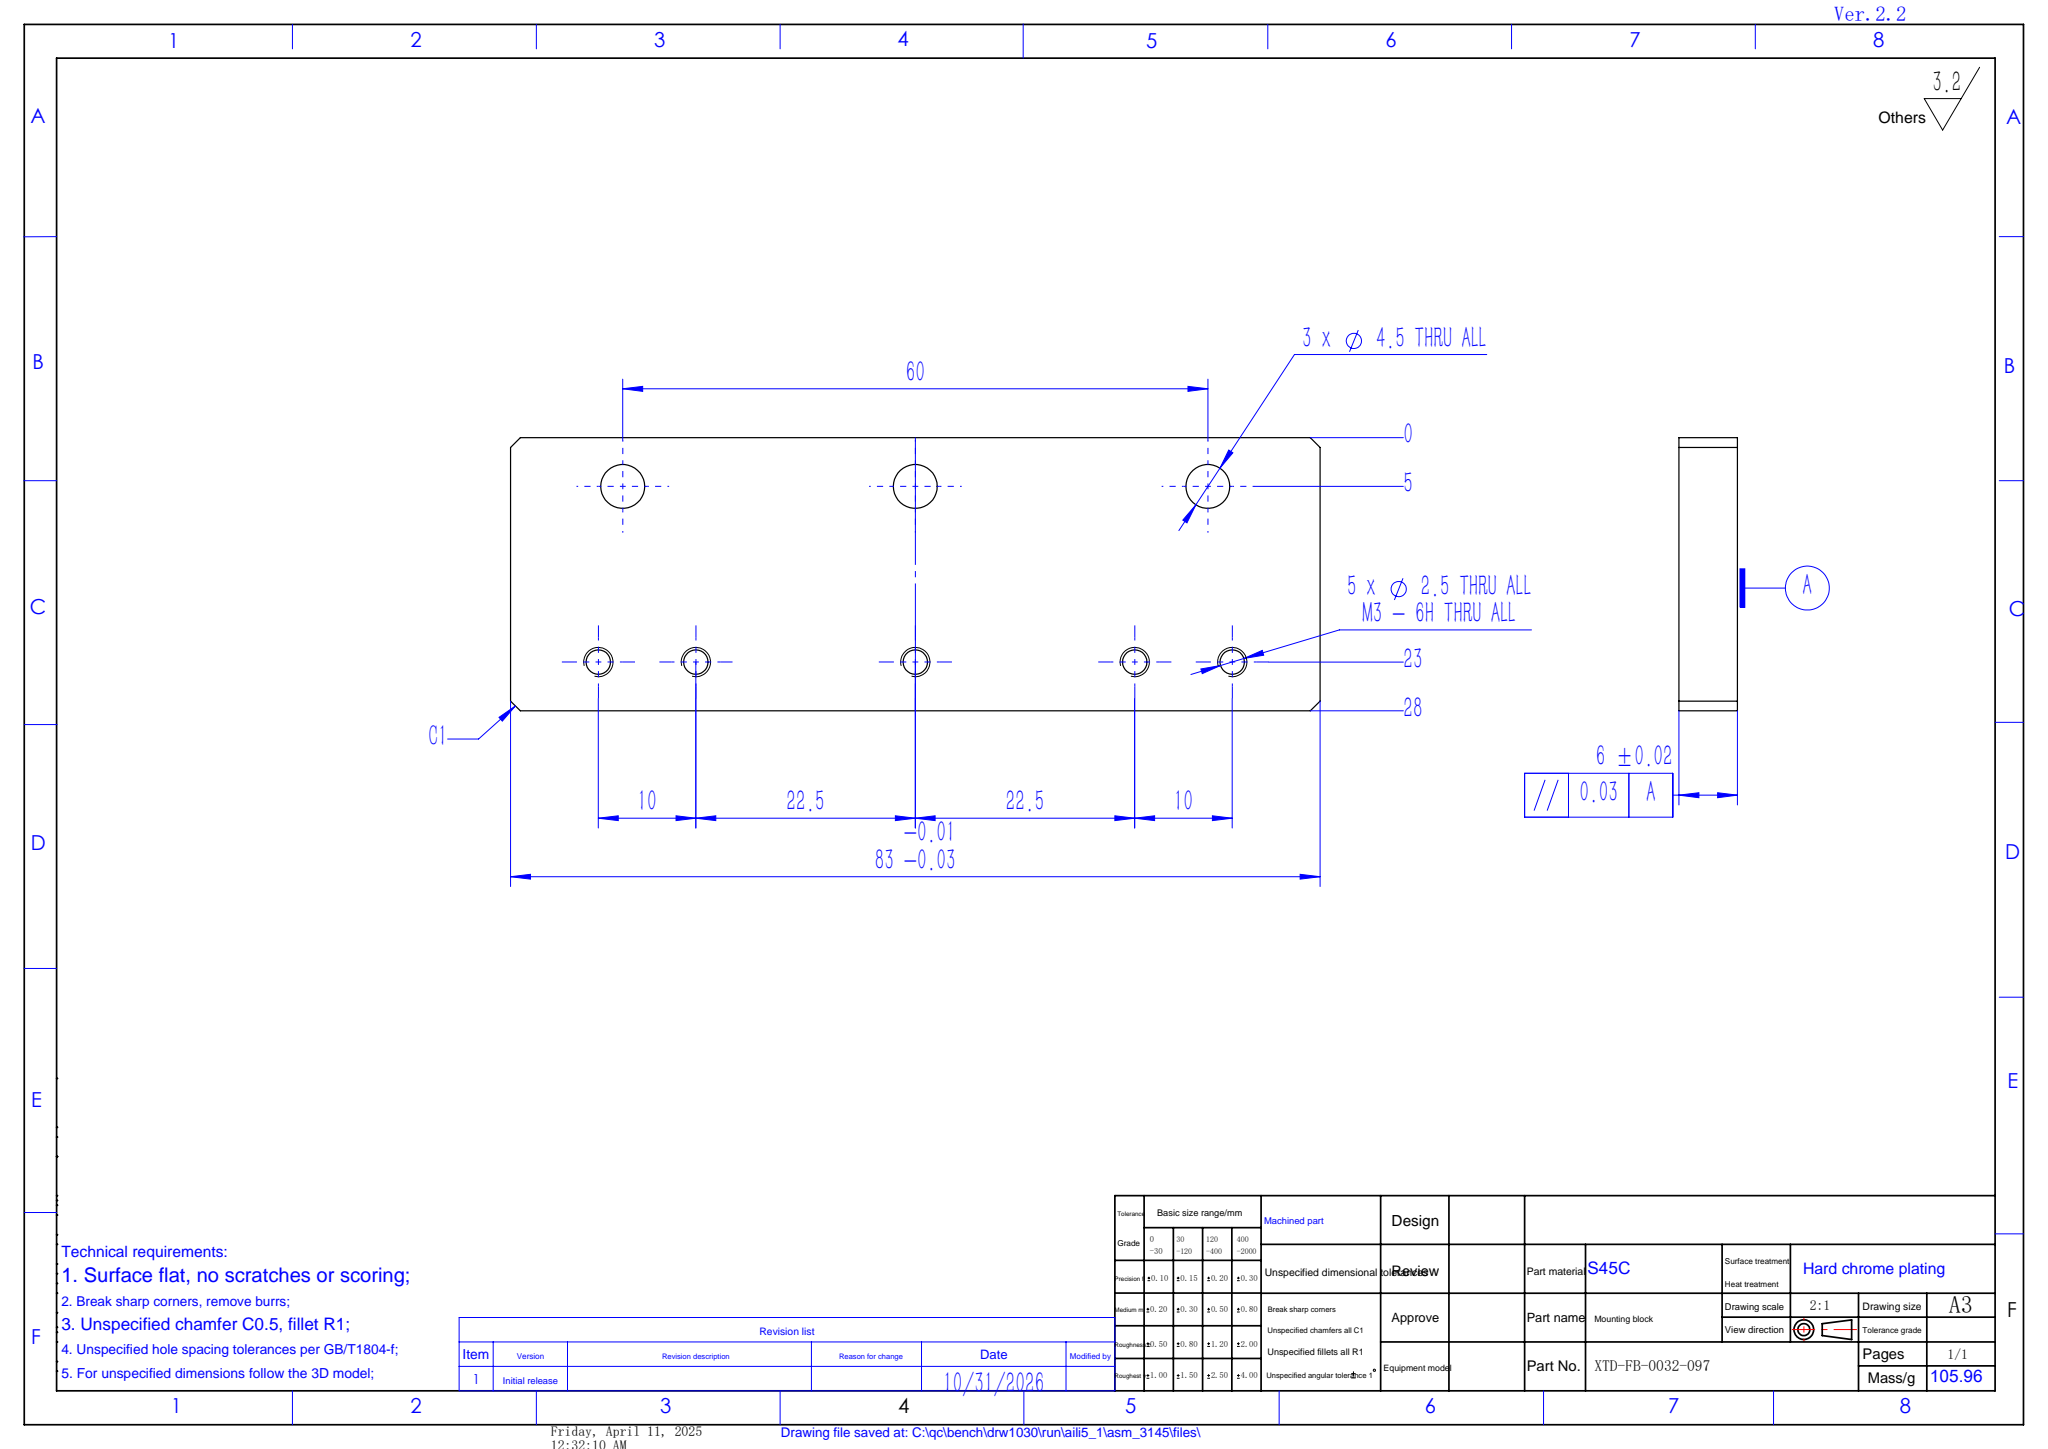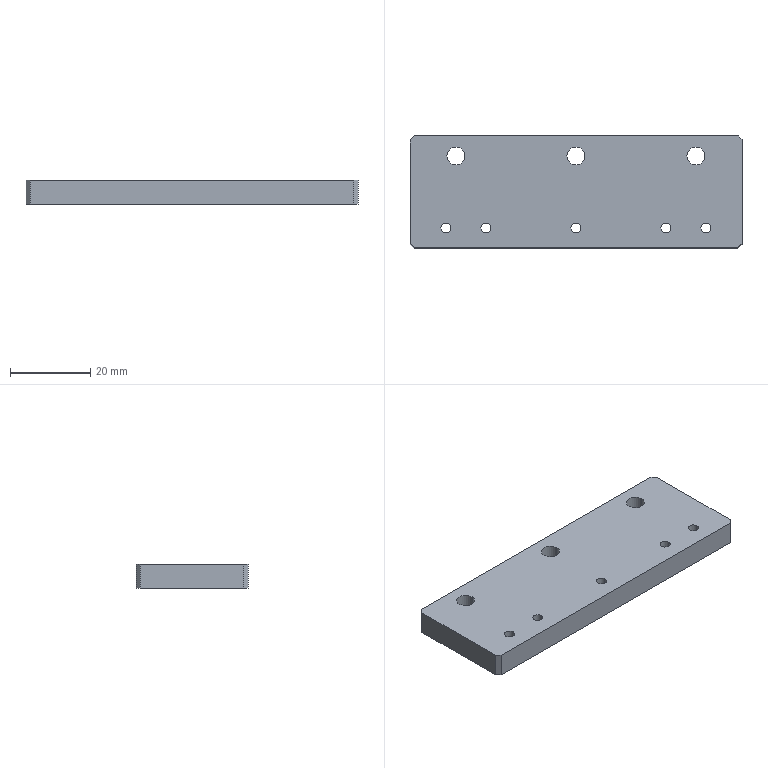Part | SolidWorks | features HoleWzd 2, Chamfer 1, Extrusion 1 | 1 solid | 26 faces | box 83 x 28 x 6 mm | volume 13498 mm3 | cylinder 16 | plane 10 | commonest cylinder face diameters 2.5 x10 4.5 x6
STEP:
#1=CARTESIAN_POINT('',(-33.75,-9.,0.));
#2=VERTEX_POINT('',#1);
#3=CARTESIAN_POINT('',(-31.25,-9.,0.));
#4=VERTEX_POINT('',#3);
#5=CARTESIAN_POINT('',(-32.5,-9.,0.));
#6=DIRECTION('',(0.,0.,1.));
#7=DIRECTION('',(1.,0.,0.));
#8=AXIS2_PLACEMENT_3D('',#5,#6,#7);
#9=CIRCLE('',#8,1.25);
#10=EDGE_CURVE('',#2,#4,#9,.T.);
#11=ORIENTED_EDGE('',*,*,#10,.F.);
#12=CARTESIAN_POINT('',(-33.75,-9.,6.));
#13=VERTEX_POINT('',#12);
#14=CARTESIAN_POINT('',(-33.75,-9.,6.));
#15=DIRECTION('',(0.,0.,1.));
#16=VECTOR('',#15,1000.);
#17=LINE('',#14,#16);
#18=EDGE_CURVE('',#2,#13,#17,.T.);
#19=ORIENTED_EDGE('',*,*,#18,.T.);
#20=CARTESIAN_POINT('',(-31.25,-9.,6.));
#21=VERTEX_POINT('',#20);
#22=CARTESIAN_POINT('',(-32.5,-9.,6.));
#23=DIRECTION('',(0.,0.,1.));
#24=DIRECTION('',(1.,0.,0.));
#25=AXIS2_PLACEMENT_3D('',#22,#23,#24);
#26=CIRCLE('',#25,1.25);
#27=EDGE_CURVE('',#13,#21,#26,.T.);
#28=ORIENTED_EDGE('',*,*,#27,.T.);
#29=CARTESIAN_POINT('',(-31.25,-9.,6.));
#30=DIRECTION('',(0.,0.,1.));
#31=VECTOR('',#30,1000.);
#32=LINE('',#29,#31);
#33=EDGE_CURVE('',#4,#21,#32,.T.);
#34=ORIENTED_EDGE('',*,*,#33,.F.);
#35=EDGE_LOOP('',(#11,#19,#28,#34));
#36=FACE_OUTER_BOUND('',#35,.T.);
#37=CARTESIAN_POINT('',(-32.5,-9.,6.));
#38=DIRECTION('',(0.,0.,1.));
#39=DIRECTION('',(1.,0.,0.));
#40=AXIS2_PLACEMENT_3D('',#37,#38,#39);
#41=CYLINDRICAL_SURFACE('',#40,1.25);
#42=ADVANCED_FACE('',(#36),#41,.F.);
#43=CARTESIAN_POINT('',(-1.25,-9.,0.));
#44=VERTEX_POINT('',#43);
#45=CARTESIAN_POINT('',(1.25,-9.,0.));
#46=VERTEX_POINT('',#45);
#47=CARTESIAN_POINT('',(0.,-9.,0.));
#48=DIRECTION('',(0.,0.,1.));
#49=DIRECTION('',(1.,0.,0.));
#50=AXIS2_PLACEMENT_3D('',#47,#48,#49);
#51=CIRCLE('',#50,1.25);
#52=EDGE_CURVE('',#44,#46,#51,.T.);
#53=ORIENTED_EDGE('',*,*,#52,.F.);
#54=CARTESIAN_POINT('',(-1.25,-9.,6.));
#55=VERTEX_POINT('',#54);
#56=CARTESIAN_POINT('',(-1.25,-9.,6.));
#57=DIRECTION('',(0.,0.,1.));
#58=VECTOR('',#57,1000.);
#59=LINE('',#56,#58);
#60=EDGE_CURVE('',#44,#55,#59,.T.);
#61=ORIENTED_EDGE('',*,*,#60,.T.);
#62=CARTESIAN_POINT('',(1.25,-9.,6.));
#63=VERTEX_POINT('',#62);
#64=CARTESIAN_POINT('',(0.,-9.,6.));
#65=DIRECTION('',(0.,0.,1.));
#66=DIRECTION('',(1.,0.,0.));
#67=AXIS2_PLACEMENT_3D('',#64,#65,#66);
#68=CIRCLE('',#67,1.25);
#69=EDGE_CURVE('',#55,#63,#68,.T.);
#70=ORIENTED_EDGE('',*,*,#69,.T.);
#71=CARTESIAN_POINT('',(1.25,-9.,6.));
#72=DIRECTION('',(0.,0.,1.));
#73=VECTOR('',#72,1000.);
#74=LINE('',#71,#73);
#75=EDGE_CURVE('',#46,#63,#74,.T.);
#76=ORIENTED_EDGE('',*,*,#75,.F.);
#77=EDGE_LOOP('',(#53,#61,#70,#76));
#78=FACE_OUTER_BOUND('',#77,.T.);
#79=CARTESIAN_POINT('',(0.,-9.,6.));
#80=DIRECTION('',(0.,0.,1.));
#81=DIRECTION('',(1.,0.,0.));
#82=AXIS2_PLACEMENT_3D('',#79,#80,#81);
#83=CYLINDRICAL_SURFACE('',#82,1.25);
#84=ADVANCED_FACE('',(#78),#83,.F.);
#85=CARTESIAN_POINT('',(31.25,-9.,0.));
#86=VERTEX_POINT('',#85);
#87=CARTESIAN_POINT('',(33.75,-9.,0.));
#88=VERTEX_POINT('',#87);
#89=CARTESIAN_POINT('',(32.5,-9.,0.));
#90=DIRECTION('',(0.,0.,1.));
#91=DIRECTION('',(1.,0.,0.));
#92=AXIS2_PLACEMENT_3D('',#89,#90,#91);
#93=CIRCLE('',#92,1.25);
#94=EDGE_CURVE('',#86,#88,#93,.T.);
#95=ORIENTED_EDGE('',*,*,#94,.F.);
#96=CARTESIAN_POINT('',(31.25,-9.,6.));
#97=VERTEX_POINT('',#96);
#98=CARTESIAN_POINT('',(31.25,-9.,6.));
#99=DIRECTION('',(0.,0.,1.));
#100=VECTOR('',#99,1000.);
#101=LINE('',#98,#100);
#102=EDGE_CURVE('',#86,#97,#101,.T.);
#103=ORIENTED_EDGE('',*,*,#102,.T.);
#104=CARTESIAN_POINT('',(33.75,-9.,6.));
#105=VERTEX_POINT('',#104);
#106=CARTESIAN_POINT('',(32.5,-9.,6.));
#107=DIRECTION('',(0.,0.,1.));
#108=DIRECTION('',(1.,0.,0.));
#109=AXIS2_PLACEMENT_3D('',#106,#107,#108);
#110=CIRCLE('',#109,1.25);
#111=EDGE_CURVE('',#97,#105,#110,.T.);
#112=ORIENTED_EDGE('',*,*,#111,.T.);
#113=CARTESIAN_POINT('',(33.75,-9.,6.));
#114=DIRECTION('',(0.,0.,1.));
#115=VECTOR('',#114,1000.);
#116=LINE('',#113,#115);
#117=EDGE_CURVE('',#88,#105,#116,.T.);
#118=ORIENTED_EDGE('',*,*,#117,.F.);
#119=EDGE_LOOP('',(#95,#103,#112,#118));
#120=FACE_OUTER_BOUND('',#119,.T.);
#121=CARTESIAN_POINT('',(32.5,-9.,6.));
#122=DIRECTION('',(0.,0.,1.));
#123=DIRECTION('',(1.,0.,0.));
#124=AXIS2_PLACEMENT_3D('',#121,#122,#123);
#125=CYLINDRICAL_SURFACE('',#124,1.25);
#126=ADVANCED_FACE('',(#120),#125,.F.);
#127=CARTESIAN_POINT('',(21.25,-9.,0.));
#128=VERTEX_POINT('',#127);
#129=CARTESIAN_POINT('',(23.75,-9.,0.));
#130=VERTEX_POINT('',#129);
#131=CARTESIAN_POINT('',(22.5,-9.,0.));
#132=DIRECTION('',(0.,0.,1.));
#133=DIRECTION('',(1.,0.,0.));
#134=AXIS2_PLACEMENT_3D('',#131,#132,#133);
#135=CIRCLE('',#134,1.25);
#136=EDGE_CURVE('',#128,#130,#135,.T.);
#137=ORIENTED_EDGE('',*,*,#136,.F.);
#138=CARTESIAN_POINT('',(21.25,-9.,6.));
#139=VERTEX_POINT('',#138);
#140=CARTESIAN_POINT('',(21.25,-9.,6.));
#141=DIRECTION('',(0.,0.,1.));
#142=VECTOR('',#141,1000.);
#143=LINE('',#140,#142);
#144=EDGE_CURVE('',#128,#139,#143,.T.);
#145=ORIENTED_EDGE('',*,*,#144,.T.);
#146=CARTESIAN_POINT('',(23.75,-9.,6.));
#147=VERTEX_POINT('',#146);
#148=CARTESIAN_POINT('',(22.5,-9.,6.));
#149=DIRECTION('',(0.,0.,1.));
#150=DIRECTION('',(1.,0.,0.));
#151=AXIS2_PLACEMENT_3D('',#148,#149,#150);
#152=CIRCLE('',#151,1.25);
#153=EDGE_CURVE('',#139,#147,#152,.T.);
#154=ORIENTED_EDGE('',*,*,#153,.T.);
#155=CARTESIAN_POINT('',(23.75,-9.,6.));
#156=DIRECTION('',(0.,0.,1.));
#157=VECTOR('',#156,1000.);
#158=LINE('',#155,#157);
#159=EDGE_CURVE('',#130,#147,#158,.T.);
#160=ORIENTED_EDGE('',*,*,#159,.F.);
#161=EDGE_LOOP('',(#137,#145,#154,#160));
#162=FACE_OUTER_BOUND('',#161,.T.);
#163=CARTESIAN_POINT('',(22.5,-9.,6.));
#164=DIRECTION('',(0.,0.,1.));
#165=DIRECTION('',(1.,0.,0.));
#166=AXIS2_PLACEMENT_3D('',#163,#164,#165);
#167=CYLINDRICAL_SURFACE('',#166,1.25);
#168=ADVANCED_FACE('',(#162),#167,.F.);
#169=CARTESIAN_POINT('',(-23.75,-9.,0.));
#170=VERTEX_POINT('',#169);
#171=CARTESIAN_POINT('',(-21.25,-9.,0.));
#172=VERTEX_POINT('',#171);
#173=CARTESIAN_POINT('',(-22.5,-9.,0.));
#174=DIRECTION('',(0.,0.,1.));
#175=DIRECTION('',(1.,0.,0.));
#176=AXIS2_PLACEMENT_3D('',#173,#174,#175);
#177=CIRCLE('',#176,1.25);
#178=EDGE_CURVE('',#170,#172,#177,.T.);
#179=ORIENTED_EDGE('',*,*,#178,.F.);
#180=CARTESIAN_POINT('',(-23.75,-9.,6.));
#181=VERTEX_POINT('',#180);
#182=CARTESIAN_POINT('',(-23.75,-9.,6.));
#183=DIRECTION('',(0.,0.,1.));
#184=VECTOR('',#183,1000.);
#185=LINE('',#182,#184);
#186=EDGE_CURVE('',#170,#181,#185,.T.);
#187=ORIENTED_EDGE('',*,*,#186,.T.);
#188=CARTESIAN_POINT('',(-21.25,-9.,6.));
#189=VERTEX_POINT('',#188);
#190=CARTESIAN_POINT('',(-22.5,-9.,6.));
#191=DIRECTION('',(0.,0.,1.));
#192=DIRECTION('',(1.,0.,0.));
#193=AXIS2_PLACEMENT_3D('',#190,#191,#192);
#194=CIRCLE('',#193,1.25);
#195=EDGE_CURVE('',#181,#189,#194,.T.);
#196=ORIENTED_EDGE('',*,*,#195,.T.);
#197=CARTESIAN_POINT('',(-21.25,-9.,6.));
#198=DIRECTION('',(0.,0.,1.));
#199=VECTOR('',#198,1000.);
#200=LINE('',#197,#199);
#201=EDGE_CURVE('',#172,#189,#200,.T.);
#202=ORIENTED_EDGE('',*,*,#201,.F.);
#203=EDGE_LOOP('',(#179,#187,#196,#202));
#204=FACE_OUTER_BOUND('',#203,.T.);
#205=CARTESIAN_POINT('',(-22.5,-9.,6.));
#206=DIRECTION('',(0.,0.,1.));
#207=DIRECTION('',(1.,0.,0.));
#208=AXIS2_PLACEMENT_3D('',#205,#206,#207);
#209=CYLINDRICAL_SURFACE('',#208,1.25);
#210=ADVANCED_FACE('',(#204),#209,.F.);
#211=CARTESIAN_POINT('',(-32.25,9.,0.));
#212=VERTEX_POINT('',#211);
#213=CARTESIAN_POINT('',(-27.75,9.,0.));
#214=VERTEX_POINT('',#213);
#215=CARTESIAN_POINT('',(-30.,9.,0.));
#216=DIRECTION('',(0.,0.,1.));
#217=DIRECTION('',(1.,0.,0.));
#218=AXIS2_PLACEMENT_3D('',#215,#216,#217);
#219=CIRCLE('',#218,2.25);
#220=EDGE_CURVE('',#212,#214,#219,.T.);
#221=ORIENTED_EDGE('',*,*,#220,.F.);
#222=CARTESIAN_POINT('',(-32.25,9.,6.));
#223=VERTEX_POINT('',#222);
#224=CARTESIAN_POINT('',(-32.25,9.,6.));
#225=DIRECTION('',(0.,0.,1.));
#226=VECTOR('',#225,1000.);
#227=LINE('',#224,#226);
#228=EDGE_CURVE('',#212,#223,#227,.T.);
#229=ORIENTED_EDGE('',*,*,#228,.T.);
#230=CARTESIAN_POINT('',(-27.75,9.,6.));
#231=VERTEX_POINT('',#230);
#232=CARTESIAN_POINT('',(-30.,9.,6.));
#233=DIRECTION('',(0.,0.,1.));
#234=DIRECTION('',(1.,0.,0.));
#235=AXIS2_PLACEMENT_3D('',#232,#233,#234);
#236=CIRCLE('',#235,2.25);
#237=EDGE_CURVE('',#223,#231,#236,.T.);
#238=ORIENTED_EDGE('',*,*,#237,.T.);
#239=CARTESIAN_POINT('',(-27.75,9.,6.));
#240=DIRECTION('',(0.,0.,1.));
#241=VECTOR('',#240,1000.);
#242=LINE('',#239,#241);
#243=EDGE_CURVE('',#214,#231,#242,.T.);
#244=ORIENTED_EDGE('',*,*,#243,.F.);
#245=EDGE_LOOP('',(#221,#229,#238,#244));
#246=FACE_OUTER_BOUND('',#245,.T.);
#247=CARTESIAN_POINT('',(-30.,9.,6.));
#248=DIRECTION('',(0.,0.,1.));
#249=DIRECTION('',(1.,0.,0.));
#250=AXIS2_PLACEMENT_3D('',#247,#248,#249);
#251=CYLINDRICAL_SURFACE('',#250,2.25);
#252=ADVANCED_FACE('',(#246),#251,.F.);
#253=CARTESIAN_POINT('',(-2.25,9.,0.));
#254=VERTEX_POINT('',#253);
#255=CARTESIAN_POINT('',(2.25,9.,0.));
#256=VERTEX_POINT('',#255);
#257=CARTESIAN_POINT('',(0.,9.,0.));
#258=DIRECTION('',(0.,0.,1.));
#259=DIRECTION('',(1.,0.,0.));
#260=AXIS2_PLACEMENT_3D('',#257,#258,#259);
#261=CIRCLE('',#260,2.25);
#262=EDGE_CURVE('',#254,#256,#261,.T.);
#263=ORIENTED_EDGE('',*,*,#262,.F.);
#264=CARTESIAN_POINT('',(-2.25,9.,6.));
#265=VERTEX_POINT('',#264);
#266=CARTESIAN_POINT('',(-2.25,9.,6.));
#267=DIRECTION('',(0.,0.,1.));
#268=VECTOR('',#267,1000.);
#269=LINE('',#266,#268);
#270=EDGE_CURVE('',#254,#265,#269,.T.);
#271=ORIENTED_EDGE('',*,*,#270,.T.);
#272=CARTESIAN_POINT('',(2.25,9.,6.));
#273=VERTEX_POINT('',#272);
#274=CARTESIAN_POINT('',(0.,9.,6.));
#275=DIRECTION('',(0.,0.,1.));
#276=DIRECTION('',(1.,0.,0.));
#277=AXIS2_PLACEMENT_3D('',#274,#275,#276);
#278=CIRCLE('',#277,2.25);
#279=EDGE_CURVE('',#265,#273,#278,.T.);
#280=ORIENTED_EDGE('',*,*,#279,.T.);
#281=CARTESIAN_POINT('',(2.25,9.,6.));
#282=DIRECTION('',(0.,0.,1.));
#283=VECTOR('',#282,1000.);
#284=LINE('',#281,#283);
#285=EDGE_CURVE('',#256,#273,#284,.T.);
#286=ORIENTED_EDGE('',*,*,#285,.F.);
#287=EDGE_LOOP('',(#263,#271,#280,#286));
#288=FACE_OUTER_BOUND('',#287,.T.);
#289=CARTESIAN_POINT('',(0.,9.,6.));
#290=DIRECTION('',(0.,0.,1.));
#291=DIRECTION('',(1.,0.,0.));
#292=AXIS2_PLACEMENT_3D('',#289,#290,#291);
#293=CYLINDRICAL_SURFACE('',#292,2.25);
#294=ADVANCED_FACE('',(#288),#293,.F.);
#295=CARTESIAN_POINT('',(27.75,9.,0.));
#296=VERTEX_POINT('',#295);
#297=CARTESIAN_POINT('',(32.25,9.,0.));
#298=VERTEX_POINT('',#297);
#299=CARTESIAN_POINT('',(30.,9.,0.));
#300=DIRECTION('',(0.,0.,1.));
#301=DIRECTION('',(1.,0.,0.));
#302=AXIS2_PLACEMENT_3D('',#299,#300,#301);
#303=CIRCLE('',#302,2.25);
#304=EDGE_CURVE('',#296,#298,#303,.T.);
#305=ORIENTED_EDGE('',*,*,#304,.F.);
#306=CARTESIAN_POINT('',(27.75,9.,6.));
#307=VERTEX_POINT('',#306);
#308=CARTESIAN_POINT('',(27.75,9.,6.));
#309=DIRECTION('',(0.,0.,1.));
#310=VECTOR('',#309,1000.);
#311=LINE('',#308,#310);
#312=EDGE_CURVE('',#296,#307,#311,.T.);
#313=ORIENTED_EDGE('',*,*,#312,.T.);
#314=CARTESIAN_POINT('',(32.25,9.,6.));
#315=VERTEX_POINT('',#314);
#316=CARTESIAN_POINT('',(30.,9.,6.));
#317=DIRECTION('',(0.,0.,1.));
#318=DIRECTION('',(1.,0.,0.));
#319=AXIS2_PLACEMENT_3D('',#316,#317,#318);
#320=CIRCLE('',#319,2.25);
#321=EDGE_CURVE('',#307,#315,#320,.T.);
#322=ORIENTED_EDGE('',*,*,#321,.T.);
#323=CARTESIAN_POINT('',(32.25,9.,6.));
#324=DIRECTION('',(0.,0.,1.));
#325=VECTOR('',#324,1000.);
#326=LINE('',#323,#325);
#327=EDGE_CURVE('',#298,#315,#326,.T.);
#328=ORIENTED_EDGE('',*,*,#327,.F.);
#329=EDGE_LOOP('',(#305,#313,#322,#328));
#330=FACE_OUTER_BOUND('',#329,.T.);
#331=CARTESIAN_POINT('',(30.,9.,6.));
#332=DIRECTION('',(0.,0.,1.));
#333=DIRECTION('',(1.,0.,0.));
#334=AXIS2_PLACEMENT_3D('',#331,#332,#333);
#335=CYLINDRICAL_SURFACE('',#334,2.25);
#336=ADVANCED_FACE('',(#330),#335,.F.);
#337=CARTESIAN_POINT('',(41.5,-13.,0.));
#338=VERTEX_POINT('',#337);
#339=CARTESIAN_POINT('',(41.5,13.,0.));
#340=VERTEX_POINT('',#339);
#341=CARTESIAN_POINT('',(41.5,14.,0.));
#342=DIRECTION('',(0.,1.,0.));
#343=VECTOR('',#342,1000.);
#344=LINE('',#341,#343);
#345=EDGE_CURVE('',#338,#340,#344,.T.);
#346=ORIENTED_EDGE('',*,*,#345,.T.);
#347=CARTESIAN_POINT('',(41.5,13.,6.));
#348=VERTEX_POINT('',#347);
#349=CARTESIAN_POINT('',(41.5,13.,6.));
#350=DIRECTION('',(0.,0.,1.));
#351=VECTOR('',#350,1000.);
#352=LINE('',#349,#351);
#353=EDGE_CURVE('',#340,#348,#352,.T.);
#354=ORIENTED_EDGE('',*,*,#353,.T.);
#355=CARTESIAN_POINT('',(41.5,-13.,6.));
#356=VERTEX_POINT('',#355);
#357=CARTESIAN_POINT('',(41.5,14.,6.));
#358=DIRECTION('',(0.,1.,0.));
#359=VECTOR('',#358,1000.);
#360=LINE('',#357,#359);
#361=EDGE_CURVE('',#356,#348,#360,.T.);
#362=ORIENTED_EDGE('',*,*,#361,.F.);
#363=CARTESIAN_POINT('',(41.5,-13.,6.));
#364=DIRECTION('',(0.,0.,-1.));
#365=VECTOR('',#364,1000.);
#366=LINE('',#363,#365);
#367=EDGE_CURVE('',#356,#338,#366,.T.);
#368=ORIENTED_EDGE('',*,*,#367,.T.);
#369=EDGE_LOOP('',(#346,#354,#362,#368));
#370=FACE_OUTER_BOUND('',#369,.T.);
#371=CARTESIAN_POINT('',(41.5,14.,6.));
#372=DIRECTION('',(-1.,0.,0.));
#373=DIRECTION('',(0.,-1.,0.));
#374=AXIS2_PLACEMENT_3D('',#371,#372,#373);
#375=PLANE('',#374);
#376=ADVANCED_FACE('',(#370),#375,.F.);
#377=CARTESIAN_POINT('',(40.5,14.,6.));
#378=VERTEX_POINT('',#377);
#379=CARTESIAN_POINT('',(-40.5,14.,6.));
#380=VERTEX_POINT('',#379);
#381=CARTESIAN_POINT('',(-41.5,14.,6.));
#382=DIRECTION('',(-1.,0.,0.));
#383=VECTOR('',#382,1000.);
#384=LINE('',#381,#383);
#385=EDGE_CURVE('',#378,#380,#384,.T.);
#386=ORIENTED_EDGE('',*,*,#385,.F.);
#387=CARTESIAN_POINT('',(40.5,14.,0.));
#388=VERTEX_POINT('',#387);
#389=CARTESIAN_POINT('',(40.5,14.,6.));
#390=DIRECTION('',(0.,0.,-1.));
#391=VECTOR('',#390,1000.);
#392=LINE('',#389,#391);
#393=EDGE_CURVE('',#378,#388,#392,.T.);
#394=ORIENTED_EDGE('',*,*,#393,.T.);
#395=CARTESIAN_POINT('',(-40.5,14.,0.));
#396=VERTEX_POINT('',#395);
#397=CARTESIAN_POINT('',(-41.5,14.,0.));
#398=DIRECTION('',(-1.,0.,0.));
#399=VECTOR('',#398,1000.);
#400=LINE('',#397,#399);
#401=EDGE_CURVE('',#388,#396,#400,.T.);
#402=ORIENTED_EDGE('',*,*,#401,.T.);
#403=CARTESIAN_POINT('',(-40.5,14.,6.));
#404=DIRECTION('',(0.,0.,1.));
#405=VECTOR('',#404,1000.);
#406=LINE('',#403,#405);
#407=EDGE_CURVE('',#396,#380,#406,.T.);
#408=ORIENTED_EDGE('',*,*,#407,.T.);
#409=EDGE_LOOP('',(#386,#394,#402,#408));
#410=FACE_OUTER_BOUND('',#409,.T.);
#411=CARTESIAN_POINT('',(-41.5,14.,6.));
#412=DIRECTION('',(0.,-1.,0.));
#413=DIRECTION('',(0.,0.,-1.));
#414=AXIS2_PLACEMENT_3D('',#411,#412,#413);
#415=PLANE('',#414);
#416=ADVANCED_FACE('',(#410),#415,.F.);
#417=CARTESIAN_POINT('',(-41.5,13.,0.));
#418=VERTEX_POINT('',#417);
#419=CARTESIAN_POINT('',(-41.5,-13.,0.));
#420=VERTEX_POINT('',#419);
#421=CARTESIAN_POINT('',(-41.5,14.,0.));
#422=DIRECTION('',(0.,-1.,0.));
#423=VECTOR('',#422,1000.);
#424=LINE('',#421,#423);
#425=EDGE_CURVE('',#418,#420,#424,.T.);
#426=ORIENTED_EDGE('',*,*,#425,.T.);
#427=CARTESIAN_POINT('',(-41.5,-13.,6.));
#428=VERTEX_POINT('',#427);
#429=CARTESIAN_POINT('',(-41.5,-13.,6.));
#430=DIRECTION('',(0.,0.,1.));
#431=VECTOR('',#430,1000.);
#432=LINE('',#429,#431);
#433=EDGE_CURVE('',#420,#428,#432,.T.);
#434=ORIENTED_EDGE('',*,*,#433,.T.);
#435=CARTESIAN_POINT('',(-41.5,13.,6.));
#436=VERTEX_POINT('',#435);
#437=CARTESIAN_POINT('',(-41.5,14.,6.));
#438=DIRECTION('',(0.,-1.,0.));
#439=VECTOR('',#438,1000.);
#440=LINE('',#437,#439);
#441=EDGE_CURVE('',#436,#428,#440,.T.);
#442=ORIENTED_EDGE('',*,*,#441,.F.);
#443=CARTESIAN_POINT('',(-41.5,13.,6.));
#444=DIRECTION('',(0.,0.,-1.));
#445=VECTOR('',#444,1000.);
#446=LINE('',#443,#445);
#447=EDGE_CURVE('',#436,#418,#446,.T.);
#448=ORIENTED_EDGE('',*,*,#447,.T.);
#449=EDGE_LOOP('',(#426,#434,#442,#448));
#450=FACE_OUTER_BOUND('',#449,.T.);
#451=CARTESIAN_POINT('',(-41.5,14.,6.));
#452=DIRECTION('',(1.,0.,0.));
#453=DIRECTION('',(0.,0.,-1.));
#454=AXIS2_PLACEMENT_3D('',#451,#452,#453);
#455=PLANE('',#454);
#456=ADVANCED_FACE('',(#450),#455,.F.);
#457=CARTESIAN_POINT('',(-40.5,-14.,0.));
#458=VERTEX_POINT('',#457);
#459=CARTESIAN_POINT('',(40.5,-14.,0.));
#460=VERTEX_POINT('',#459);
#461=CARTESIAN_POINT('',(-41.5,-14.,0.));
#462=DIRECTION('',(1.,0.,0.));
#463=VECTOR('',#462,1000.);
#464=LINE('',#461,#463);
#465=EDGE_CURVE('',#458,#460,#464,.T.);
#466=ORIENTED_EDGE('',*,*,#465,.T.);
#467=CARTESIAN_POINT('',(40.5,-14.,6.));
#468=VERTEX_POINT('',#467);
#469=CARTESIAN_POINT('',(40.5,-14.,6.));
#470=DIRECTION('',(0.,0.,1.));
#471=VECTOR('',#470,1000.);
#472=LINE('',#469,#471);
#473=EDGE_CURVE('',#460,#468,#472,.T.);
#474=ORIENTED_EDGE('',*,*,#473,.T.);
#475=CARTESIAN_POINT('',(-40.5,-14.,6.));
#476=VERTEX_POINT('',#475);
#477=CARTESIAN_POINT('',(-41.5,-14.,6.));
#478=DIRECTION('',(1.,0.,0.));
#479=VECTOR('',#478,1000.);
#480=LINE('',#477,#479);
#481=EDGE_CURVE('',#476,#468,#480,.T.);
#482=ORIENTED_EDGE('',*,*,#481,.F.);
#483=CARTESIAN_POINT('',(-40.5,-14.,6.));
#484=DIRECTION('',(0.,0.,-1.));
#485=VECTOR('',#484,1000.);
#486=LINE('',#483,#485);
#487=EDGE_CURVE('',#476,#458,#486,.T.);
#488=ORIENTED_EDGE('',*,*,#487,.T.);
#489=EDGE_LOOP('',(#466,#474,#482,#488));
#490=FACE_OUTER_BOUND('',#489,.T.);
#491=CARTESIAN_POINT('',(-41.5,-14.,6.));
#492=DIRECTION('',(0.,1.,0.));
#493=DIRECTION('',(0.,0.,1.));
#494=AXIS2_PLACEMENT_3D('',#491,#492,#493);
#495=PLANE('',#494);
#496=ADVANCED_FACE('',(#490),#495,.F.);
#497=CARTESIAN_POINT('',(-32.5,-9.,6.));
#498=DIRECTION('',(0.,0.,1.));
#499=DIRECTION('',(1.,0.,0.));
#500=AXIS2_PLACEMENT_3D('',#497,#498,#499);
#501=CIRCLE('',#500,1.25);
#502=EDGE_CURVE('',#21,#13,#501,.T.);
#503=ORIENTED_EDGE('',*,*,#502,.F.);
#504=ORIENTED_EDGE('',*,*,#27,.F.);
#505=EDGE_LOOP('',(#503,#504));
#506=FACE_BOUND('',#505,.T.);
#507=CARTESIAN_POINT('',(0.,-9.,6.));
#508=DIRECTION('',(0.,0.,1.));
#509=DIRECTION('',(1.,0.,0.));
#510=AXIS2_PLACEMENT_3D('',#507,#508,#509);
#511=CIRCLE('',#510,1.25);
#512=EDGE_CURVE('',#63,#55,#511,.T.);
#513=ORIENTED_EDGE('',*,*,#512,.F.);
#514=ORIENTED_EDGE('',*,*,#69,.F.);
#515=EDGE_LOOP('',(#513,#514));
#516=FACE_BOUND('',#515,.T.);
#517=CARTESIAN_POINT('',(32.5,-9.,6.));
#518=DIRECTION('',(0.,0.,1.));
#519=DIRECTION('',(1.,0.,0.));
#520=AXIS2_PLACEMENT_3D('',#517,#518,#519);
#521=CIRCLE('',#520,1.25);
#522=EDGE_CURVE('',#105,#97,#521,.T.);
#523=ORIENTED_EDGE('',*,*,#522,.F.);
#524=ORIENTED_EDGE('',*,*,#111,.F.);
#525=EDGE_LOOP('',(#523,#524));
#526=FACE_BOUND('',#525,.T.);
#527=CARTESIAN_POINT('',(22.5,-9.,6.));
#528=DIRECTION('',(0.,0.,1.));
#529=DIRECTION('',(1.,0.,0.));
#530=AXIS2_PLACEMENT_3D('',#527,#528,#529);
#531=CIRCLE('',#530,1.25);
#532=EDGE_CURVE('',#147,#139,#531,.T.);
#533=ORIENTED_EDGE('',*,*,#532,.F.);
#534=ORIENTED_EDGE('',*,*,#153,.F.);
#535=EDGE_LOOP('',(#533,#534));
#536=FACE_BOUND('',#535,.T.);
#537=CARTESIAN_POINT('',(-22.5,-9.,6.));
#538=DIRECTION('',(0.,0.,1.));
#539=DIRECTION('',(1.,0.,0.));
#540=AXIS2_PLACEMENT_3D('',#537,#538,#539);
#541=CIRCLE('',#540,1.25);
#542=EDGE_CURVE('',#189,#181,#541,.T.);
#543=ORIENTED_EDGE('',*,*,#542,.F.);
#544=ORIENTED_EDGE('',*,*,#195,.F.);
#545=EDGE_LOOP('',(#543,#544));
#546=FACE_BOUND('',#545,.T.);
#547=CARTESIAN_POINT('',(-30.,9.,6.));
#548=DIRECTION('',(0.,0.,1.));
#549=DIRECTION('',(1.,0.,0.));
#550=AXIS2_PLACEMENT_3D('',#547,#548,#549);
#551=CIRCLE('',#550,2.25);
#552=EDGE_CURVE('',#231,#223,#551,.T.);
#553=ORIENTED_EDGE('',*,*,#552,.F.);
#554=ORIENTED_EDGE('',*,*,#237,.F.);
#555=EDGE_LOOP('',(#553,#554));
#556=FACE_BOUND('',#555,.T.);
#557=CARTESIAN_POINT('',(0.,9.,6.));
#558=DIRECTION('',(0.,0.,1.));
#559=DIRECTION('',(1.,0.,0.));
#560=AXIS2_PLACEMENT_3D('',#557,#558,#559);
#561=CIRCLE('',#560,2.25);
#562=EDGE_CURVE('',#273,#265,#561,.T.);
#563=ORIENTED_EDGE('',*,*,#562,.F.);
#564=ORIENTED_EDGE('',*,*,#279,.F.);
#565=EDGE_LOOP('',(#563,#564));
#566=FACE_BOUND('',#565,.T.);
#567=CARTESIAN_POINT('',(30.,9.,6.));
#568=DIRECTION('',(0.,0.,1.));
#569=DIRECTION('',(1.,0.,0.));
#570=AXIS2_PLACEMENT_3D('',#567,#568,#569);
#571=CIRCLE('',#570,2.25);
#572=EDGE_CURVE('',#315,#307,#571,.T.);
#573=ORIENTED_EDGE('',*,*,#572,.F.);
#574=ORIENTED_EDGE('',*,*,#321,.F.);
#575=EDGE_LOOP('',(#573,#574));
#576=FACE_BOUND('',#575,.T.);
#577=ORIENTED_EDGE('',*,*,#361,.T.);
#578=CARTESIAN_POINT('',(27.25,27.25,6.));
#579=DIRECTION('',(-0.7071,0.7071,0.));
#580=VECTOR('',#579,1000.);
#581=LINE('',#578,#580);
#582=EDGE_CURVE('',#348,#378,#581,.T.);
#583=ORIENTED_EDGE('',*,*,#582,.T.);
#584=ORIENTED_EDGE('',*,*,#385,.T.);
#585=CARTESIAN_POINT('',(-27.25,27.25,6.));
#586=DIRECTION('',(-0.7071,-0.7071,0.));
#587=VECTOR('',#586,1000.);
#588=LINE('',#585,#587);
#589=EDGE_CURVE('',#380,#436,#588,.T.);
#590=ORIENTED_EDGE('',*,*,#589,.T.);
#591=ORIENTED_EDGE('',*,*,#441,.T.);
#592=CARTESIAN_POINT('',(-27.25,-27.25,6.));
#593=DIRECTION('',(0.7071,-0.7071,0.));
#594=VECTOR('',#593,1000.);
#595=LINE('',#592,#594);
#596=EDGE_CURVE('',#428,#476,#595,.T.);
#597=ORIENTED_EDGE('',*,*,#596,.T.);
#598=ORIENTED_EDGE('',*,*,#481,.T.);
#599=CARTESIAN_POINT('',(27.25,-27.25,6.));
#600=DIRECTION('',(0.7071,0.7071,0.));
#601=VECTOR('',#600,1000.);
#602=LINE('',#599,#601);
#603=EDGE_CURVE('',#468,#356,#602,.T.);
#604=ORIENTED_EDGE('',*,*,#603,.T.);
#605=EDGE_LOOP('',(#577,#583,#584,#590,#591,#597,#598,#604));
#606=FACE_OUTER_BOUND('',#605,.T.);
#607=CARTESIAN_POINT('',(0.,0.,6.));
#608=DIRECTION('',(0.,0.,1.));
#609=DIRECTION('',(1.,0.,0.));
#610=AXIS2_PLACEMENT_3D('',#607,#608,#609);
#611=PLANE('',#610);
#612=ADVANCED_FACE('',(#506,#516,#526,#536,#546,#556,#566,#576,#606),#611,.T.);
#613=CARTESIAN_POINT('',(-32.5,-9.,0.));
#614=DIRECTION('',(0.,0.,1.));
#615=DIRECTION('',(1.,0.,0.));
#616=AXIS2_PLACEMENT_3D('',#613,#614,#615);
#617=CIRCLE('',#616,1.25);
#618=EDGE_CURVE('',#4,#2,#617,.T.);
#619=ORIENTED_EDGE('',*,*,#618,.T.);
#620=ORIENTED_EDGE('',*,*,#10,.T.);
#621=EDGE_LOOP('',(#619,#620));
#622=FACE_BOUND('',#621,.T.);
#623=CARTESIAN_POINT('',(0.,-9.,0.));
#624=DIRECTION('',(0.,0.,1.));
#625=DIRECTION('',(1.,0.,0.));
#626=AXIS2_PLACEMENT_3D('',#623,#624,#625);
#627=CIRCLE('',#626,1.25);
#628=EDGE_CURVE('',#46,#44,#627,.T.);
#629=ORIENTED_EDGE('',*,*,#628,.T.);
#630=ORIENTED_EDGE('',*,*,#52,.T.);
#631=EDGE_LOOP('',(#629,#630));
#632=FACE_BOUND('',#631,.T.);
#633=CARTESIAN_POINT('',(32.5,-9.,0.));
#634=DIRECTION('',(0.,0.,1.));
#635=DIRECTION('',(1.,0.,0.));
#636=AXIS2_PLACEMENT_3D('',#633,#634,#635);
#637=CIRCLE('',#636,1.25);
#638=EDGE_CURVE('',#88,#86,#637,.T.);
#639=ORIENTED_EDGE('',*,*,#638,.T.);
#640=ORIENTED_EDGE('',*,*,#94,.T.);
#641=EDGE_LOOP('',(#639,#640));
#642=FACE_BOUND('',#641,.T.);
#643=CARTESIAN_POINT('',(22.5,-9.,0.));
#644=DIRECTION('',(0.,0.,1.));
#645=DIRECTION('',(1.,0.,0.));
#646=AXIS2_PLACEMENT_3D('',#643,#644,#645);
#647=CIRCLE('',#646,1.25);
#648=EDGE_CURVE('',#130,#128,#647,.T.);
#649=ORIENTED_EDGE('',*,*,#648,.T.);
#650=ORIENTED_EDGE('',*,*,#136,.T.);
#651=EDGE_LOOP('',(#649,#650));
#652=FACE_BOUND('',#651,.T.);
#653=CARTESIAN_POINT('',(-22.5,-9.,0.));
#654=DIRECTION('',(0.,0.,1.));
#655=DIRECTION('',(1.,0.,0.));
#656=AXIS2_PLACEMENT_3D('',#653,#654,#655);
#657=CIRCLE('',#656,1.25);
#658=EDGE_CURVE('',#172,#170,#657,.T.);
#659=ORIENTED_EDGE('',*,*,#658,.T.);
#660=ORIENTED_EDGE('',*,*,#178,.T.);
#661=EDGE_LOOP('',(#659,#660));
#662=FACE_BOUND('',#661,.T.);
#663=CARTESIAN_POINT('',(-30.,9.,0.));
#664=DIRECTION('',(0.,0.,1.));
#665=DIRECTION('',(1.,0.,0.));
#666=AXIS2_PLACEMENT_3D('',#663,#664,#665);
#667=CIRCLE('',#666,2.25);
#668=EDGE_CURVE('',#214,#212,#667,.T.);
#669=ORIENTED_EDGE('',*,*,#668,.T.);
#670=ORIENTED_EDGE('',*,*,#220,.T.);
#671=EDGE_LOOP('',(#669,#670));
#672=FACE_BOUND('',#671,.T.);
#673=CARTESIAN_POINT('',(0.,9.,0.));
#674=DIRECTION('',(0.,0.,1.));
#675=DIRECTION('',(1.,0.,0.));
#676=AXIS2_PLACEMENT_3D('',#673,#674,#675);
#677=CIRCLE('',#676,2.25);
#678=EDGE_CURVE('',#256,#254,#677,.T.);
#679=ORIENTED_EDGE('',*,*,#678,.T.);
#680=ORIENTED_EDGE('',*,*,#262,.T.);
#681=EDGE_LOOP('',(#679,#680));
#682=FACE_BOUND('',#681,.T.);
#683=CARTESIAN_POINT('',(30.,9.,0.));
#684=DIRECTION('',(0.,0.,1.));
#685=DIRECTION('',(1.,0.,0.));
#686=AXIS2_PLACEMENT_3D('',#683,#684,#685);
#687=CIRCLE('',#686,2.25);
#688=EDGE_CURVE('',#298,#296,#687,.T.);
#689=ORIENTED_EDGE('',*,*,#688,.T.);
#690=ORIENTED_EDGE('',*,*,#304,.T.);
#691=EDGE_LOOP('',(#689,#690));
#692=FACE_BOUND('',#691,.T.);
#693=ORIENTED_EDGE('',*,*,#401,.F.);
#694=CARTESIAN_POINT('',(40.5,14.,0.));
#695=DIRECTION('',(0.7071,-0.7071,0.));
#696=VECTOR('',#695,1000.);
#697=LINE('',#694,#696);
#698=EDGE_CURVE('',#388,#340,#697,.T.);
#699=ORIENTED_EDGE('',*,*,#698,.T.);
#700=ORIENTED_EDGE('',*,*,#345,.F.);
#701=CARTESIAN_POINT('',(41.5,-13.,0.));
#702=DIRECTION('',(-0.7071,-0.7071,0.));
#703=VECTOR('',#702,1000.);
#704=LINE('',#701,#703);
#705=EDGE_CURVE('',#338,#460,#704,.T.);
#706=ORIENTED_EDGE('',*,*,#705,.T.);
#707=ORIENTED_EDGE('',*,*,#465,.F.);
#708=CARTESIAN_POINT('',(-40.5,-14.,0.));
#709=DIRECTION('',(-0.7071,0.7071,0.));
#710=VECTOR('',#709,1000.);
#711=LINE('',#708,#710);
#712=EDGE_CURVE('',#458,#420,#711,.T.);
#713=ORIENTED_EDGE('',*,*,#712,.T.);
#714=ORIENTED_EDGE('',*,*,#425,.F.);
#715=CARTESIAN_POINT('',(-41.5,13.,0.));
#716=DIRECTION('',(0.7071,0.7071,0.));
#717=VECTOR('',#716,1000.);
#718=LINE('',#715,#717);
#719=EDGE_CURVE('',#418,#396,#718,.T.);
#720=ORIENTED_EDGE('',*,*,#719,.T.);
#721=EDGE_LOOP('',(#693,#699,#700,#706,#707,#713,#714,#720));
#722=FACE_OUTER_BOUND('',#721,.T.);
#723=CARTESIAN_POINT('',(0.,0.,0.));
#724=DIRECTION('',(0.,0.,1.));
#725=DIRECTION('',(1.,0.,0.));
#726=AXIS2_PLACEMENT_3D('',#723,#724,#725);
#727=PLANE('',#726);
#728=ADVANCED_FACE('',(#622,#632,#642,#652,#662,#672,#682,#692,#722),#727,.F.);
#729=ORIENTED_EDGE('',*,*,#312,.F.);
#730=ORIENTED_EDGE('',*,*,#688,.F.);
#731=ORIENTED_EDGE('',*,*,#327,.T.);
#732=ORIENTED_EDGE('',*,*,#572,.T.);
#733=EDGE_LOOP('',(#729,#730,#731,#732));
#734=FACE_OUTER_BOUND('',#733,.T.);
#735=CARTESIAN_POINT('',(30.,9.,6.));
#736=DIRECTION('',(0.,0.,1.));
#737=DIRECTION('',(1.,0.,0.));
#738=AXIS2_PLACEMENT_3D('',#735,#736,#737);
#739=CYLINDRICAL_SURFACE('',#738,2.25);
#740=ADVANCED_FACE('',(#734),#739,.F.);
#741=ORIENTED_EDGE('',*,*,#270,.F.);
#742=ORIENTED_EDGE('',*,*,#678,.F.);
#743=ORIENTED_EDGE('',*,*,#285,.T.);
#744=ORIENTED_EDGE('',*,*,#562,.T.);
#745=EDGE_LOOP('',(#741,#742,#743,#744));
#746=FACE_OUTER_BOUND('',#745,.T.);
#747=CARTESIAN_POINT('',(0.,9.,6.));
#748=DIRECTION('',(0.,0.,1.));
#749=DIRECTION('',(1.,0.,0.));
#750=AXIS2_PLACEMENT_3D('',#747,#748,#749);
#751=CYLINDRICAL_SURFACE('',#750,2.25);
#752=ADVANCED_FACE('',(#746),#751,.F.);
#753=ORIENTED_EDGE('',*,*,#228,.F.);
#754=ORIENTED_EDGE('',*,*,#668,.F.);
#755=ORIENTED_EDGE('',*,*,#243,.T.);
#756=ORIENTED_EDGE('',*,*,#552,.T.);
#757=EDGE_LOOP('',(#753,#754,#755,#756));
#758=FACE_OUTER_BOUND('',#757,.T.);
#759=CARTESIAN_POINT('',(-30.,9.,6.));
#760=DIRECTION('',(0.,0.,1.));
#761=DIRECTION('',(1.,0.,0.));
#762=AXIS2_PLACEMENT_3D('',#759,#760,#761);
#763=CYLINDRICAL_SURFACE('',#762,2.25);
#764=ADVANCED_FACE('',(#758),#763,.F.);
#765=ORIENTED_EDGE('',*,*,#186,.F.);
#766=ORIENTED_EDGE('',*,*,#658,.F.);
#767=ORIENTED_EDGE('',*,*,#201,.T.);
#768=ORIENTED_EDGE('',*,*,#542,.T.);
#769=EDGE_LOOP('',(#765,#766,#767,#768));
#770=FACE_OUTER_BOUND('',#769,.T.);
#771=CARTESIAN_POINT('',(-22.5,-9.,6.));
#772=DIRECTION('',(0.,0.,1.));
#773=DIRECTION('',(1.,0.,0.));
#774=AXIS2_PLACEMENT_3D('',#771,#772,#773);
#775=CYLINDRICAL_SURFACE('',#774,1.25);
#776=ADVANCED_FACE('',(#770),#775,.F.);
#777=ORIENTED_EDGE('',*,*,#144,.F.);
#778=ORIENTED_EDGE('',*,*,#648,.F.);
#779=ORIENTED_EDGE('',*,*,#159,.T.);
#780=ORIENTED_EDGE('',*,*,#532,.T.);
#781=EDGE_LOOP('',(#777,#778,#779,#780));
#782=FACE_OUTER_BOUND('',#781,.T.);
#783=CARTESIAN_POINT('',(22.5,-9.,6.));
#784=DIRECTION('',(0.,0.,1.));
#785=DIRECTION('',(1.,0.,0.));
#786=AXIS2_PLACEMENT_3D('',#783,#784,#785);
#787=CYLINDRICAL_SURFACE('',#786,1.25);
#788=ADVANCED_FACE('',(#782),#787,.F.);
#789=ORIENTED_EDGE('',*,*,#102,.F.);
#790=ORIENTED_EDGE('',*,*,#638,.F.);
#791=ORIENTED_EDGE('',*,*,#117,.T.);
#792=ORIENTED_EDGE('',*,*,#522,.T.);
#793=EDGE_LOOP('',(#789,#790,#791,#792));
#794=FACE_OUTER_BOUND('',#793,.T.);
#795=CARTESIAN_POINT('',(32.5,-9.,6.));
#796=DIRECTION('',(0.,0.,1.));
#797=DIRECTION('',(1.,0.,0.));
#798=AXIS2_PLACEMENT_3D('',#795,#796,#797);
#799=CYLINDRICAL_SURFACE('',#798,1.25);
#800=ADVANCED_FACE('',(#794),#799,.F.);
#801=ORIENTED_EDGE('',*,*,#60,.F.);
#802=ORIENTED_EDGE('',*,*,#628,.F.);
#803=ORIENTED_EDGE('',*,*,#75,.T.);
#804=ORIENTED_EDGE('',*,*,#512,.T.);
#805=EDGE_LOOP('',(#801,#802,#803,#804));
#806=FACE_OUTER_BOUND('',#805,.T.);
#807=CARTESIAN_POINT('',(0.,-9.,6.));
#808=DIRECTION('',(0.,0.,1.));
#809=DIRECTION('',(1.,0.,0.));
#810=AXIS2_PLACEMENT_3D('',#807,#808,#809);
#811=CYLINDRICAL_SURFACE('',#810,1.25);
#812=ADVANCED_FACE('',(#806),#811,.F.);
#813=ORIENTED_EDGE('',*,*,#18,.F.);
#814=ORIENTED_EDGE('',*,*,#618,.F.);
#815=ORIENTED_EDGE('',*,*,#33,.T.);
#816=ORIENTED_EDGE('',*,*,#502,.T.);
#817=EDGE_LOOP('',(#813,#814,#815,#816));
#818=FACE_OUTER_BOUND('',#817,.T.);
#819=CARTESIAN_POINT('',(-32.5,-9.,6.));
#820=DIRECTION('',(0.,0.,1.));
#821=DIRECTION('',(1.,0.,0.));
#822=AXIS2_PLACEMENT_3D('',#819,#820,#821);
#823=CYLINDRICAL_SURFACE('',#822,1.25);
#824=ADVANCED_FACE('',(#818),#823,.F.);
#825=ORIENTED_EDGE('',*,*,#582,.F.);
#826=ORIENTED_EDGE('',*,*,#353,.F.);
#827=ORIENTED_EDGE('',*,*,#698,.F.);
#828=ORIENTED_EDGE('',*,*,#393,.F.);
#829=EDGE_LOOP('',(#825,#826,#827,#828));
#830=FACE_OUTER_BOUND('',#829,.T.);
#831=CARTESIAN_POINT('',(40.5,14.,6.));
#832=DIRECTION('',(-0.7071,-0.7071,0.));
#833=DIRECTION('',(0.,0.,-1.));
#834=AXIS2_PLACEMENT_3D('',#831,#832,#833);
#835=PLANE('',#834);
#836=ADVANCED_FACE('',(#830),#835,.F.);
#837=ORIENTED_EDGE('',*,*,#603,.F.);
#838=ORIENTED_EDGE('',*,*,#473,.F.);
#839=ORIENTED_EDGE('',*,*,#705,.F.);
#840=ORIENTED_EDGE('',*,*,#367,.F.);
#841=EDGE_LOOP('',(#837,#838,#839,#840));
#842=FACE_OUTER_BOUND('',#841,.T.);
#843=CARTESIAN_POINT('',(41.5,-13.,6.));
#844=DIRECTION('',(-0.7071,0.7071,0.));
#845=DIRECTION('',(0.,0.,-1.));
#846=AXIS2_PLACEMENT_3D('',#843,#844,#845);
#847=PLANE('',#846);
#848=ADVANCED_FACE('',(#842),#847,.F.);
#849=ORIENTED_EDGE('',*,*,#596,.F.);
#850=ORIENTED_EDGE('',*,*,#433,.F.);
#851=ORIENTED_EDGE('',*,*,#712,.F.);
#852=ORIENTED_EDGE('',*,*,#487,.F.);
#853=EDGE_LOOP('',(#849,#850,#851,#852));
#854=FACE_OUTER_BOUND('',#853,.T.);
#855=CARTESIAN_POINT('',(-40.5,-14.,6.));
#856=DIRECTION('',(0.7071,0.7071,0.));
#857=DIRECTION('',(0.,0.,-1.));
#858=AXIS2_PLACEMENT_3D('',#855,#856,#857);
#859=PLANE('',#858);
#860=ADVANCED_FACE('',(#854),#859,.F.);
#861=ORIENTED_EDGE('',*,*,#589,.F.);
#862=ORIENTED_EDGE('',*,*,#407,.F.);
#863=ORIENTED_EDGE('',*,*,#719,.F.);
#864=ORIENTED_EDGE('',*,*,#447,.F.);
#865=EDGE_LOOP('',(#861,#862,#863,#864));
#866=FACE_OUTER_BOUND('',#865,.T.);
#867=CARTESIAN_POINT('',(-41.5,13.,6.));
#868=DIRECTION('',(0.7071,-0.7071,0.));
#869=DIRECTION('',(0.,0.,-1.));
#870=AXIS2_PLACEMENT_3D('',#867,#868,#869);
#871=PLANE('',#870);
#872=ADVANCED_FACE('',(#866),#871,.F.);
#873=CLOSED_SHELL('',(#42,#84,#126,#168,#210,#252,#294,#336,#376,#416,#456,#496,#612,#728,#740,#752,#764,#776,#788,#800,#812,#824,#836,#848,#860,#872));
#874=MANIFOLD_SOLID_BREP('',#873);
#875=CARTESIAN_POINT('',(0.,0.,0.));
#876=DIRECTION('',(0.,0.,1.));
#877=DIRECTION('',(1.,0.,0.));
#878=AXIS2_PLACEMENT_3D('',#875,#876,#877);
#879=(LENGTH_UNIT()NAMED_UNIT(*)SI_UNIT(.MILLI.,.METRE.));
#880=UNCERTAINTY_MEASURE_WITH_UNIT(LENGTH_MEASURE(0.00001),#879,'','');
#881=(NAMED_UNIT(*)PLANE_ANGLE_UNIT()SI_UNIT($,.RADIAN.));
#882=(NAMED_UNIT(*)SI_UNIT($,.STERADIAN.)SOLID_ANGLE_UNIT());
#883=(GEOMETRIC_REPRESENTATION_CONTEXT(3)GLOBAL_UNCERTAINTY_ASSIGNED_CONTEXT((#880))GLOBAL_UNIT_ASSIGNED_CONTEXT((#879,#881,#882))REPRESENTATION_CONTEXT('',''));
#884=ADVANCED_BREP_SHAPE_REPRESENTATION('',(#874,#878),#883);